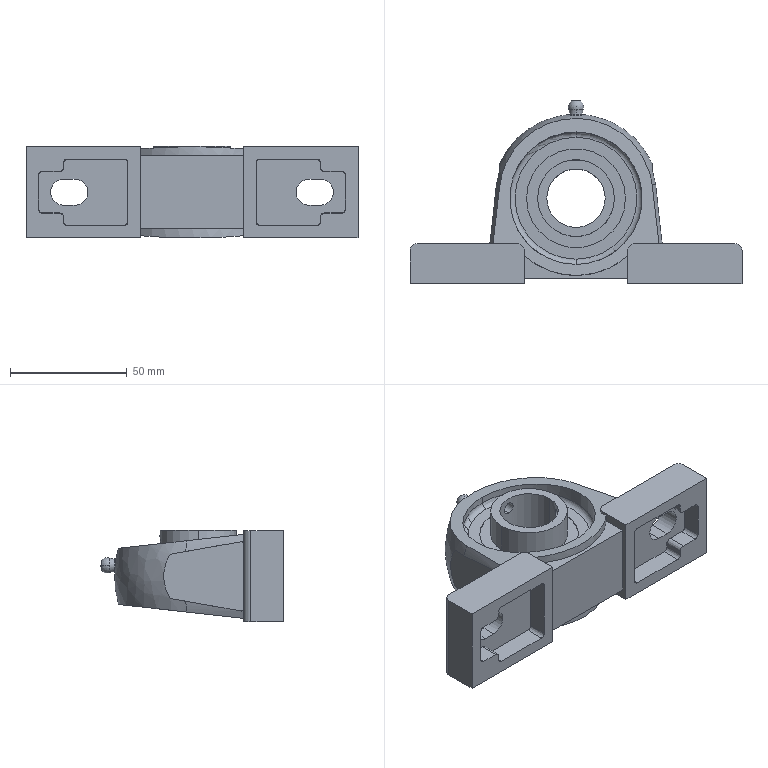Part | SolidWorks | features Revolution 5, Cut 3, Boss 2, CirPattern 2, ICE 2, RevCut 2, Extrusion 1, RefAxis 1, SweepCut 1 | 1 solid | 160 faces | box 142 x 78.36 x 39.3 mm | volume 118845 mm3 | plane 56 | cylinder 43 | sphere 32 | cone 16 | torus 8 | spline 5 | commonest cylinder face diameters 2 x6 6 x6 32.83 x6 42.32 x6 56.695 x6 5.134 x4